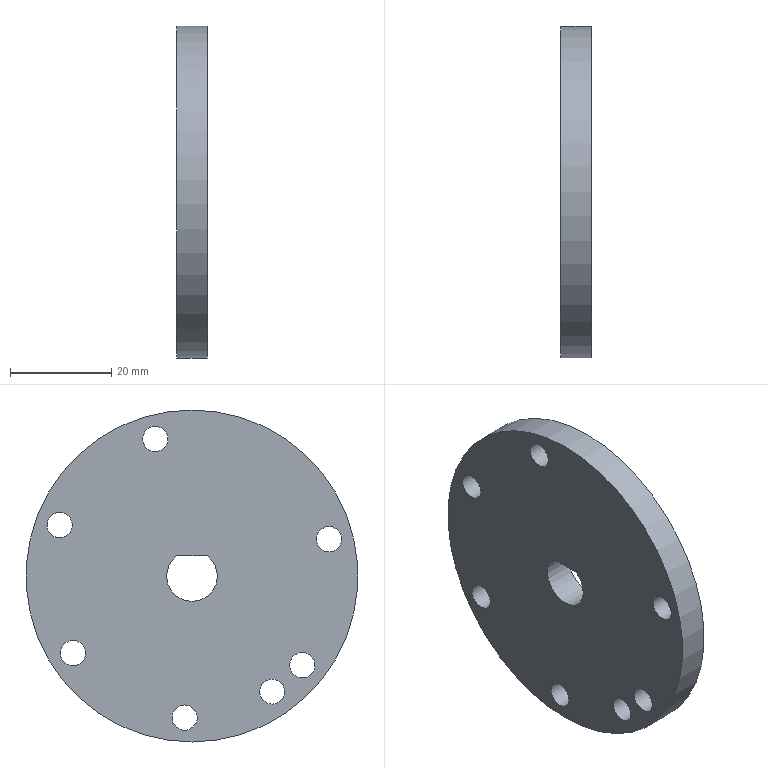Part | NX | features EXTRUDE 8, EXTRACT_FACE 6, EXTRACT_STRING 6, Instance Feature 5, DATUM_CSYS 2, SKETCH 2, HOLE PACKAGE 1, LINKED_CURVE 1, Pattern Feature 1, SIMPLE HOLE 1, SYMBOLIC_THREAD 1 | 1 solid | 12 faces | box 6 x 65.544 x 65.544 mm | volume 18977 mm3 | cylinder 9 | plane 3 | commonest cylinder face diameters 5 x6 4.917 x1 10 x1 65.544 x1
STEP:
#1=CARTESIAN_POINT('',(6.,8.878,-32.772));
#2=VERTEX_POINT('',#1);
#3=CARTESIAN_POINT('',(6.,8.878,0.));
#4=DIRECTION('',(1.,0.,0.));
#5=DIRECTION('',(0.,0.,-1.));
#6=AXIS2_PLACEMENT_3D('',#3,#4,#5);
#7=CIRCLE('',#6,32.772);
#8=EDGE_CURVE('',#2,#2,#7,.T.);
#9=ORIENTED_EDGE('',*,*,#8,.F.);
#10=EDGE_LOOP('',(#9));
#11=FACE_BOUND('',#10,.T.);
#12=CARTESIAN_POINT('',(0.,8.878,-32.772));
#13=VERTEX_POINT('',#12);
#14=CARTESIAN_POINT('',(0.,8.878,0.));
#15=DIRECTION('',(1.,0.,0.));
#16=DIRECTION('',(0.,0.,-1.));
#17=AXIS2_PLACEMENT_3D('',#14,#15,#16);
#18=CIRCLE('',#17,32.772);
#19=EDGE_CURVE('',#13,#13,#18,.T.);
#20=ORIENTED_EDGE('',*,*,#19,.T.);
#21=EDGE_LOOP('',(#20));
#22=FACE_BOUND('',#21,.T.);
#23=CARTESIAN_POINT('',(6.,8.878,0.));
#24=DIRECTION('',(-1.,0.,0.));
#25=DIRECTION('',(0.,0.,1.));
#26=AXIS2_PLACEMENT_3D('',#23,#24,#25);
#27=CYLINDRICAL_SURFACE('',#26,32.772);
#28=ADVANCED_FACE('',(#11,#22),#27,.T.);
#29=CARTESIAN_POINT('',(6.,16.125,24.546));
#30=VERTEX_POINT('',#29);
#31=CARTESIAN_POINT('',(6.,16.125,27.046));
#32=DIRECTION('',(1.,0.,0.));
#33=DIRECTION('',(0.,0.,-1.));
#34=AXIS2_PLACEMENT_3D('',#31,#32,#33);
#35=CIRCLE('',#34,2.5);
#36=EDGE_CURVE('',#30,#30,#35,.T.);
#37=ORIENTED_EDGE('',*,*,#36,.F.);
#38=EDGE_LOOP('',(#37));
#39=FACE_BOUND('',#38,.T.);
#40=CARTESIAN_POINT('',(6.,35.018,7.534));
#41=VERTEX_POINT('',#40);
#42=CARTESIAN_POINT('',(6.,35.018,10.034));
#43=DIRECTION('',(1.,0.,0.));
#44=DIRECTION('',(0.,0.,-1.));
#45=AXIS2_PLACEMENT_3D('',#42,#43,#44);
#46=CIRCLE('',#45,2.5);
#47=EDGE_CURVE('',#41,#41,#46,.T.);
#48=ORIENTED_EDGE('',*,*,#47,.F.);
#49=EDGE_LOOP('',(#48));
#50=FACE_BOUND('',#49,.T.);
#51=CARTESIAN_POINT('',(6.,32.361,-17.75));
#52=VERTEX_POINT('',#51);
#53=CARTESIAN_POINT('',(6.,32.361,-15.25));
#54=DIRECTION('',(1.,0.,0.));
#55=DIRECTION('',(0.,0.,-1.));
#56=AXIS2_PLACEMENT_3D('',#53,#54,#55);
#57=CIRCLE('',#56,2.5);
#58=EDGE_CURVE('',#52,#52,#57,.T.);
#59=ORIENTED_EDGE('',*,*,#58,.F.);
#60=EDGE_LOOP('',(#59));
#61=FACE_BOUND('',#60,.T.);
#62=CARTESIAN_POINT('',(6.,10.343,-30.462));
#63=VERTEX_POINT('',#62);
#64=CARTESIAN_POINT('',(6.,10.343,-27.962));
#65=DIRECTION('',(1.,0.,0.));
#66=DIRECTION('',(0.,0.,-1.));
#67=AXIS2_PLACEMENT_3D('',#64,#65,#66);
#68=CIRCLE('',#67,2.5);
#69=EDGE_CURVE('',#63,#63,#68,.T.);
#70=ORIENTED_EDGE('',*,*,#69,.F.);
#71=EDGE_LOOP('',(#70));
#72=FACE_BOUND('',#71,.T.);
#73=CARTESIAN_POINT('',(6.,-12.882,-20.121));
#74=VERTEX_POINT('',#73);
#75=CARTESIAN_POINT('',(6.,-12.882,-17.621));
#76=DIRECTION('',(1.,0.,0.));
#77=DIRECTION('',(0.,0.,-1.));
#78=AXIS2_PLACEMENT_3D('',#75,#76,#77);
#79=CIRCLE('',#78,2.5);
#80=EDGE_CURVE('',#74,#74,#79,.T.);
#81=ORIENTED_EDGE('',*,*,#80,.F.);
#82=EDGE_LOOP('',(#81));
#83=FACE_BOUND('',#82,.T.);
#84=CARTESIAN_POINT('',(6.,-18.168,4.747));
#85=VERTEX_POINT('',#84);
#86=CARTESIAN_POINT('',(6.,-18.168,7.247));
#87=DIRECTION('',(1.,0.,0.));
#88=DIRECTION('',(0.,0.,-1.));
#89=AXIS2_PLACEMENT_3D('',#86,#87,#88);
#90=CIRCLE('',#89,2.5);
#91=EDGE_CURVE('',#85,#85,#90,.T.);
#92=ORIENTED_EDGE('',*,*,#91,.F.);
#93=EDGE_LOOP('',(#92));
#94=FACE_BOUND('',#93,.T.);
#95=CARTESIAN_POINT('',(6.,-6.931,-25.292));
#96=VERTEX_POINT('',#95);
#97=CARTESIAN_POINT('',(6.,-6.931,-22.833));
#98=DIRECTION('',(1.,0.,0.));
#99=DIRECTION('',(0.,0.,-1.));
#100=AXIS2_PLACEMENT_3D('',#97,#98,#99);
#101=CIRCLE('',#100,2.458);
#102=EDGE_CURVE('',#96,#96,#101,.T.);
#103=ORIENTED_EDGE('',*,*,#102,.F.);
#104=EDGE_LOOP('',(#103));
#105=FACE_BOUND('',#104,.T.);
#106=CARTESIAN_POINT('',(6.,5.878,4.));
#107=VERTEX_POINT('',#106);
#108=CARTESIAN_POINT('',(6.,11.878,4.));
#109=VERTEX_POINT('',#108);
#110=CARTESIAN_POINT('',(6.,8.878,0.));
#111=DIRECTION('',(1.,0.,0.));
#112=DIRECTION('',(0.,0.,-1.));
#113=AXIS2_PLACEMENT_3D('',#110,#111,#112);
#114=CIRCLE('',#113,5.);
#115=EDGE_CURVE('',#107,#109,#114,.T.);
#116=ORIENTED_EDGE('',*,*,#115,.F.);
#117=CARTESIAN_POINT('',(6.,11.878,4.));
#118=DIRECTION('',(0.,-1.,0.));
#119=VECTOR('',#118,1000.);
#120=LINE('',#117,#119);
#121=EDGE_CURVE('',#109,#107,#120,.T.);
#122=ORIENTED_EDGE('',*,*,#121,.F.);
#123=EDGE_LOOP('',(#116,#122));
#124=FACE_BOUND('',#123,.T.);
#125=ORIENTED_EDGE('',*,*,#8,.T.);
#126=EDGE_LOOP('',(#125));
#127=FACE_BOUND('',#126,.T.);
#128=CARTESIAN_POINT('',(6.,8.878,0.));
#129=DIRECTION('',(1.,0.,0.));
#130=DIRECTION('',(0.,0.,-1.));
#131=AXIS2_PLACEMENT_3D('',#128,#129,#130);
#132=PLANE('',#131);
#133=ADVANCED_FACE('',(#39,#50,#61,#72,#83,#94,#105,#124,#127),#132,.T.);
#134=CARTESIAN_POINT('',(0.,16.125,24.546));
#135=VERTEX_POINT('',#134);
#136=CARTESIAN_POINT('',(0.,16.125,27.046));
#137=DIRECTION('',(1.,0.,0.));
#138=DIRECTION('',(0.,0.,-1.));
#139=AXIS2_PLACEMENT_3D('',#136,#137,#138);
#140=CIRCLE('',#139,2.5);
#141=EDGE_CURVE('',#135,#135,#140,.F.);
#142=ORIENTED_EDGE('',*,*,#141,.F.);
#143=EDGE_LOOP('',(#142));
#144=FACE_BOUND('',#143,.T.);
#145=CARTESIAN_POINT('',(0.,35.018,7.534));
#146=VERTEX_POINT('',#145);
#147=CARTESIAN_POINT('',(0.,35.018,10.034));
#148=DIRECTION('',(1.,0.,0.));
#149=DIRECTION('',(0.,0.,-1.));
#150=AXIS2_PLACEMENT_3D('',#147,#148,#149);
#151=CIRCLE('',#150,2.5);
#152=EDGE_CURVE('',#146,#146,#151,.F.);
#153=ORIENTED_EDGE('',*,*,#152,.F.);
#154=EDGE_LOOP('',(#153));
#155=FACE_BOUND('',#154,.T.);
#156=CARTESIAN_POINT('',(0.,32.361,-17.75));
#157=VERTEX_POINT('',#156);
#158=CARTESIAN_POINT('',(0.,32.361,-15.25));
#159=DIRECTION('',(1.,0.,0.));
#160=DIRECTION('',(0.,0.,-1.));
#161=AXIS2_PLACEMENT_3D('',#158,#159,#160);
#162=CIRCLE('',#161,2.5);
#163=EDGE_CURVE('',#157,#157,#162,.F.);
#164=ORIENTED_EDGE('',*,*,#163,.F.);
#165=EDGE_LOOP('',(#164));
#166=FACE_BOUND('',#165,.T.);
#167=CARTESIAN_POINT('',(0.,10.343,-30.462));
#168=VERTEX_POINT('',#167);
#169=CARTESIAN_POINT('',(0.,10.343,-27.962));
#170=DIRECTION('',(1.,0.,0.));
#171=DIRECTION('',(0.,0.,-1.));
#172=AXIS2_PLACEMENT_3D('',#169,#170,#171);
#173=CIRCLE('',#172,2.5);
#174=EDGE_CURVE('',#168,#168,#173,.F.);
#175=ORIENTED_EDGE('',*,*,#174,.F.);
#176=EDGE_LOOP('',(#175));
#177=FACE_BOUND('',#176,.T.);
#178=CARTESIAN_POINT('',(0.,-12.882,-20.121));
#179=VERTEX_POINT('',#178);
#180=CARTESIAN_POINT('',(0.,-12.882,-17.621));
#181=DIRECTION('',(1.,0.,0.));
#182=DIRECTION('',(0.,0.,-1.));
#183=AXIS2_PLACEMENT_3D('',#180,#181,#182);
#184=CIRCLE('',#183,2.5);
#185=EDGE_CURVE('',#179,#179,#184,.F.);
#186=ORIENTED_EDGE('',*,*,#185,.F.);
#187=EDGE_LOOP('',(#186));
#188=FACE_BOUND('',#187,.T.);
#189=CARTESIAN_POINT('',(0.,-18.168,4.747));
#190=VERTEX_POINT('',#189);
#191=CARTESIAN_POINT('',(0.,-18.168,7.247));
#192=DIRECTION('',(1.,0.,0.));
#193=DIRECTION('',(0.,0.,-1.));
#194=AXIS2_PLACEMENT_3D('',#191,#192,#193);
#195=CIRCLE('',#194,2.5);
#196=EDGE_CURVE('',#190,#190,#195,.F.);
#197=ORIENTED_EDGE('',*,*,#196,.F.);
#198=EDGE_LOOP('',(#197));
#199=FACE_BOUND('',#198,.T.);
#200=CARTESIAN_POINT('',(0.,-6.931,-25.292));
#201=VERTEX_POINT('',#200);
#202=CARTESIAN_POINT('',(0.,-6.931,-22.833));
#203=DIRECTION('',(1.,0.,0.));
#204=DIRECTION('',(0.,0.,-1.));
#205=AXIS2_PLACEMENT_3D('',#202,#203,#204);
#206=CIRCLE('',#205,2.458);
#207=EDGE_CURVE('',#201,#201,#206,.T.);
#208=ORIENTED_EDGE('',*,*,#207,.T.);
#209=EDGE_LOOP('',(#208));
#210=FACE_BOUND('',#209,.T.);
#211=CARTESIAN_POINT('',(0.,11.878,4.));
#212=VERTEX_POINT('',#211);
#213=CARTESIAN_POINT('',(0.,5.878,4.));
#214=VERTEX_POINT('',#213);
#215=CARTESIAN_POINT('',(0.,11.878,4.));
#216=DIRECTION('',(0.,-1.,0.));
#217=VECTOR('',#216,1000.);
#218=LINE('',#215,#217);
#219=EDGE_CURVE('',#212,#214,#218,.T.);
#220=ORIENTED_EDGE('',*,*,#219,.T.);
#221=CARTESIAN_POINT('',(0.,8.878,0.));
#222=DIRECTION('',(1.,0.,0.));
#223=DIRECTION('',(0.,1.,0.));
#224=AXIS2_PLACEMENT_3D('',#221,#222,#223);
#225=CIRCLE('',#224,5.);
#226=EDGE_CURVE('',#214,#212,#225,.T.);
#227=ORIENTED_EDGE('',*,*,#226,.T.);
#228=EDGE_LOOP('',(#220,#227));
#229=FACE_BOUND('',#228,.T.);
#230=ORIENTED_EDGE('',*,*,#19,.F.);
#231=EDGE_LOOP('',(#230));
#232=FACE_BOUND('',#231,.T.);
#233=CARTESIAN_POINT('',(0.,8.878,0.));
#234=DIRECTION('',(1.,0.,0.));
#235=DIRECTION('',(0.,0.,-1.));
#236=AXIS2_PLACEMENT_3D('',#233,#234,#235);
#237=PLANE('',#236);
#238=ADVANCED_FACE('',(#144,#155,#166,#177,#188,#199,#210,#229,#232),#237,.F.);
#239=ORIENTED_EDGE('',*,*,#121,.T.);
#240=CARTESIAN_POINT('',(6.6,5.878,4.));
#241=DIRECTION('',(-1.,0.,0.));
#242=VECTOR('',#241,1000.);
#243=LINE('',#240,#242);
#244=EDGE_CURVE('',#107,#214,#243,.T.);
#245=ORIENTED_EDGE('',*,*,#244,.T.);
#246=ORIENTED_EDGE('',*,*,#219,.F.);
#247=CARTESIAN_POINT('',(6.6,11.878,4.));
#248=DIRECTION('',(-1.,0.,0.));
#249=VECTOR('',#248,1000.);
#250=LINE('',#247,#249);
#251=EDGE_CURVE('',#212,#109,#250,.F.);
#252=ORIENTED_EDGE('',*,*,#251,.T.);
#253=EDGE_LOOP('',(#239,#245,#246,#252));
#254=FACE_BOUND('',#253,.T.);
#255=CARTESIAN_POINT('',(6.6,11.878,4.));
#256=DIRECTION('',(0.,0.,-1.));
#257=DIRECTION('',(-1.,0.,0.));
#258=AXIS2_PLACEMENT_3D('',#255,#256,#257);
#259=PLANE('',#258);
#260=ADVANCED_FACE('',(#254),#259,.T.);
#261=ORIENTED_EDGE('',*,*,#115,.T.);
#262=ORIENTED_EDGE('',*,*,#251,.F.);
#263=ORIENTED_EDGE('',*,*,#226,.F.);
#264=ORIENTED_EDGE('',*,*,#244,.F.);
#265=EDGE_LOOP('',(#261,#262,#263,#264));
#266=FACE_BOUND('',#265,.T.);
#267=CARTESIAN_POINT('',(6.6,8.878,0.));
#268=DIRECTION('',(-1.,0.,0.));
#269=DIRECTION('',(0.,0.,1.));
#270=AXIS2_PLACEMENT_3D('',#267,#268,#269);
#271=CYLINDRICAL_SURFACE('',#270,5.);
#272=ADVANCED_FACE('',(#266),#271,.F.);
#273=ORIENTED_EDGE('',*,*,#102,.T.);
#274=EDGE_LOOP('',(#273));
#275=FACE_BOUND('',#274,.T.);
#276=ORIENTED_EDGE('',*,*,#207,.F.);
#277=EDGE_LOOP('',(#276));
#278=FACE_BOUND('',#277,.T.);
#279=CARTESIAN_POINT('',(0.,-6.931,-22.833));
#280=DIRECTION('',(1.,0.,0.));
#281=DIRECTION('',(0.,0.,-1.));
#282=AXIS2_PLACEMENT_3D('',#279,#280,#281);
#283=CYLINDRICAL_SURFACE('',#282,2.458);
#284=ADVANCED_FACE('',(#275,#278),#283,.F.);
#285=ORIENTED_EDGE('',*,*,#91,.T.);
#286=EDGE_LOOP('',(#285));
#287=FACE_BOUND('',#286,.T.);
#288=ORIENTED_EDGE('',*,*,#196,.T.);
#289=EDGE_LOOP('',(#288));
#290=FACE_BOUND('',#289,.T.);
#291=CARTESIAN_POINT('',(-89.,-18.168,7.247));
#292=DIRECTION('',(1.,0.,0.));
#293=DIRECTION('',(0.,0.,-1.));
#294=AXIS2_PLACEMENT_3D('',#291,#292,#293);
#295=CYLINDRICAL_SURFACE('',#294,2.5);
#296=ADVANCED_FACE('',(#287,#290),#295,.F.);
#297=ORIENTED_EDGE('',*,*,#80,.T.);
#298=EDGE_LOOP('',(#297));
#299=FACE_BOUND('',#298,.T.);
#300=ORIENTED_EDGE('',*,*,#185,.T.);
#301=EDGE_LOOP('',(#300));
#302=FACE_BOUND('',#301,.T.);
#303=CARTESIAN_POINT('',(-89.,-12.882,-17.621));
#304=DIRECTION('',(1.,0.,0.));
#305=DIRECTION('',(0.,1.,0.));
#306=AXIS2_PLACEMENT_3D('',#303,#304,#305);
#307=CYLINDRICAL_SURFACE('',#306,2.5);
#308=ADVANCED_FACE('',(#299,#302),#307,.F.);
#309=ORIENTED_EDGE('',*,*,#69,.T.);
#310=EDGE_LOOP('',(#309));
#311=FACE_BOUND('',#310,.T.);
#312=ORIENTED_EDGE('',*,*,#174,.T.);
#313=EDGE_LOOP('',(#312));
#314=FACE_BOUND('',#313,.T.);
#315=CARTESIAN_POINT('',(-89.,10.343,-27.962));
#316=DIRECTION('',(1.,0.,0.));
#317=DIRECTION('',(0.,1.,0.));
#318=AXIS2_PLACEMENT_3D('',#315,#316,#317);
#319=CYLINDRICAL_SURFACE('',#318,2.5);
#320=ADVANCED_FACE('',(#311,#314),#319,.F.);
#321=ORIENTED_EDGE('',*,*,#58,.T.);
#322=EDGE_LOOP('',(#321));
#323=FACE_BOUND('',#322,.T.);
#324=ORIENTED_EDGE('',*,*,#163,.T.);
#325=EDGE_LOOP('',(#324));
#326=FACE_BOUND('',#325,.T.);
#327=CARTESIAN_POINT('',(-89.,32.361,-15.25));
#328=DIRECTION('',(1.,0.,0.));
#329=DIRECTION('',(0.,0.,-1.));
#330=AXIS2_PLACEMENT_3D('',#327,#328,#329);
#331=CYLINDRICAL_SURFACE('',#330,2.5);
#332=ADVANCED_FACE('',(#323,#326),#331,.F.);
#333=ORIENTED_EDGE('',*,*,#47,.T.);
#334=EDGE_LOOP('',(#333));
#335=FACE_BOUND('',#334,.T.);
#336=ORIENTED_EDGE('',*,*,#152,.T.);
#337=EDGE_LOOP('',(#336));
#338=FACE_BOUND('',#337,.T.);
#339=CARTESIAN_POINT('',(-89.,35.018,10.034));
#340=DIRECTION('',(1.,0.,0.));
#341=DIRECTION('',(0.,0.,-1.));
#342=AXIS2_PLACEMENT_3D('',#339,#340,#341);
#343=CYLINDRICAL_SURFACE('',#342,2.5);
#344=ADVANCED_FACE('',(#335,#338),#343,.F.);
#345=ORIENTED_EDGE('',*,*,#36,.T.);
#346=EDGE_LOOP('',(#345));
#347=FACE_BOUND('',#346,.T.);
#348=ORIENTED_EDGE('',*,*,#141,.T.);
#349=EDGE_LOOP('',(#348));
#350=FACE_BOUND('',#349,.T.);
#351=CARTESIAN_POINT('',(-89.,16.125,27.046));
#352=DIRECTION('',(1.,0.,0.));
#353=DIRECTION('',(0.,1.,0.));
#354=AXIS2_PLACEMENT_3D('',#351,#352,#353);
#355=CYLINDRICAL_SURFACE('',#354,2.5);
#356=ADVANCED_FACE('',(#347,#350),#355,.F.);
#357=CLOSED_SHELL('',(#28,#133,#238,#260,#272,#284,#296,#308,#320,#332,#344,#356));
#358=MANIFOLD_SOLID_BREP('',#357);
#359=(LENGTH_UNIT()NAMED_UNIT(*)SI_UNIT(.MILLI.,.METRE.));
#360=UNCERTAINTY_MEASURE_WITH_UNIT(LENGTH_MEASURE(0.00001),#359,'','');
#361=(NAMED_UNIT(*)PLANE_ANGLE_UNIT()SI_UNIT($,.RADIAN.));
#362=(NAMED_UNIT(*)SI_UNIT($,.STERADIAN.)SOLID_ANGLE_UNIT());
#363=(GEOMETRIC_REPRESENTATION_CONTEXT(3)GLOBAL_UNCERTAINTY_ASSIGNED_CONTEXT((#360))GLOBAL_UNIT_ASSIGNED_CONTEXT((#359,#361,#362))REPRESENTATION_CONTEXT('',''));
#364=ADVANCED_BREP_SHAPE_REPRESENTATION('',(#358),#363);